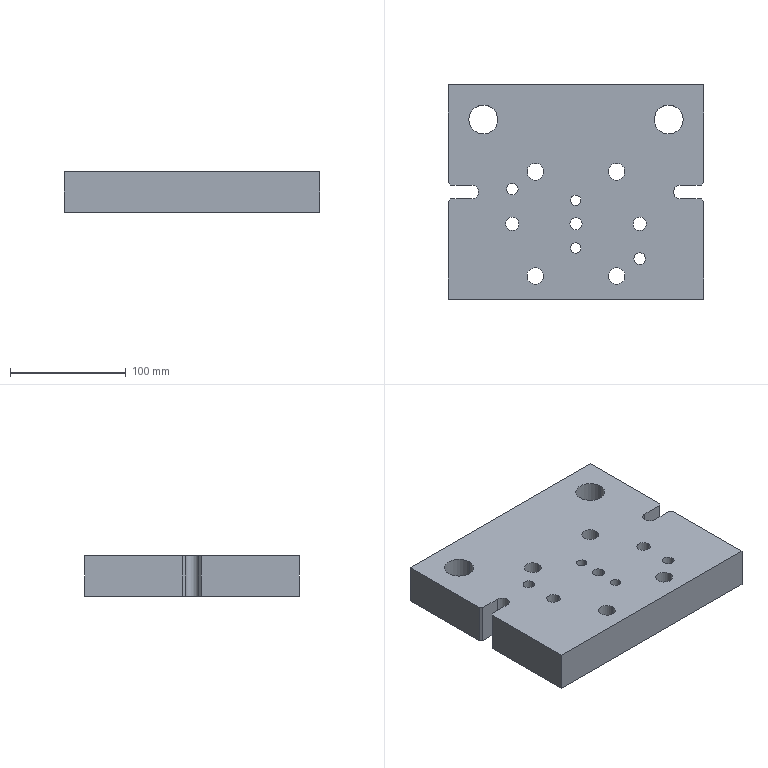Part | SolidWorks | features BaseBody 1, MoveFace 1 | 1 solid | 57 faces | box 220 x 185 x 35 mm | volume 1319567 mm3 | cylinder 37 | plane 20 | commonest cylinder face diameters 14.5 x12 9.007 x4 10 x4 11.507 x4 18 x4 25 x4